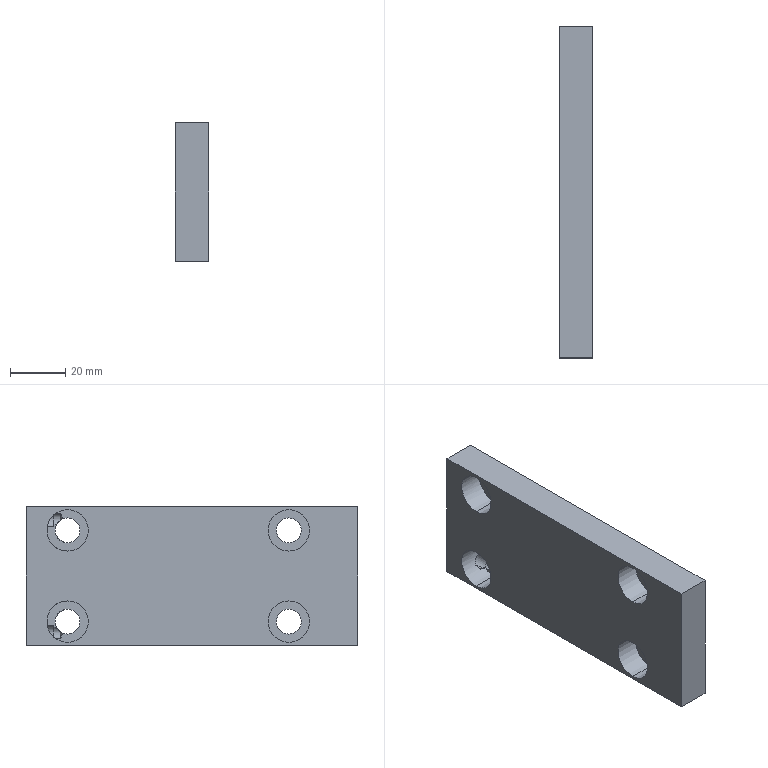Part | STEP file | X77-04102 | 1 solid | 37 faces | box 12 x 120 x 50 mm | volume 64489 mm3 | cylinder 23 | plane 12 | cone 2 | commonest cylinder face diameters 9 x8 15 x8 5 x4 4.2 x3
STEP:
#1=CARTESIAN_POINT('',(7.392,92.45,43.));
#2=VERTEX_POINT('',#1);
#3=CARTESIAN_POINT('',(5.462,90.102,47.09));
#4=VERTEX_POINT('',#3);
#5=CARTESIAN_POINT('',(7.392,92.45,43.));
#6=CARTESIAN_POINT('',(7.13,92.45,43.));
#7=CARTESIAN_POINT('',(6.865,92.442,43.042));
#8=CARTESIAN_POINT('',(6.369,92.406,43.204));
#9=CARTESIAN_POINT('',(6.131,92.378,43.325));
#10=CARTESIAN_POINT('',(5.714,92.295,43.629));
#11=CARTESIAN_POINT('',(5.528,92.239,43.815));
#12=CARTESIAN_POINT('',(5.23,92.095,44.219));
#13=CARTESIAN_POINT('',(5.113,92.005,44.443));
#14=CARTESIAN_POINT('',(4.954,91.794,44.895));
#15=CARTESIAN_POINT('',(4.909,91.671,45.128));
#16=CARTESIAN_POINT('',(4.883,91.402,45.577));
#17=CARTESIAN_POINT('',(4.9,91.254,45.797));
#18=CARTESIAN_POINT('',(4.986,90.943,46.211));
#19=CARTESIAN_POINT('',(5.052,90.782,46.404));
#20=CARTESIAN_POINT('',(5.227,90.447,46.767));
#21=CARTESIAN_POINT('',(5.335,90.274,46.936));
#22=CARTESIAN_POINT('',(5.462,90.102,47.09));
#23=B_SPLINE_CURVE_WITH_KNOTS('',3,(#5,#6,#7,#8,#9,#10,#11,#12,#13,#14,#15,#16,#17,#18,#19,#20,#21,#22),.UNSPECIFIED.,.F.,.F.,(4,2,2,2,2,2,2,2,4),(0.0005016,0.001286,0.00207,0.002854,0.003638,0.004422,0.005206,0.00599,0.006774),.UNSPECIFIED.);
#24=EDGE_CURVE('',#2,#4,#23,.T.);
#25=ORIENTED_EDGE('',*,*,#24,.F.);
#26=CARTESIAN_POINT('',(7.392,100.102,43.));
#27=VERTEX_POINT('',#26);
#28=CARTESIAN_POINT('',(7.392,100.102,43.));
#29=DIRECTION('',(0.,1.,0.));
#30=VECTOR('',#29,1000.);
#31=LINE('',#28,#30);
#32=EDGE_CURVE('',#2,#27,#31,.T.);
#33=ORIENTED_EDGE('',*,*,#32,.T.);
#34=CARTESIAN_POINT('',(7.392,100.102,48.));
#35=VERTEX_POINT('',#34);
#36=CARTESIAN_POINT('',(7.392,100.102,45.5));
#37=DIRECTION('',(0.,1.,0.));
#38=DIRECTION('',(0.,0.,1.));
#39=AXIS2_PLACEMENT_3D('',#36,#37,#38);
#40=CIRCLE('',#39,2.5);
#41=EDGE_CURVE('',#27,#35,#40,.T.);
#42=ORIENTED_EDGE('',*,*,#41,.T.);
#43=CARTESIAN_POINT('',(7.392,90.102,48.));
#44=VERTEX_POINT('',#43);
#45=CARTESIAN_POINT('',(7.392,100.102,48.));
#46=DIRECTION('',(0.,1.,0.));
#47=VECTOR('',#46,1000.);
#48=LINE('',#45,#47);
#49=EDGE_CURVE('',#44,#35,#48,.T.);
#50=ORIENTED_EDGE('',*,*,#49,.F.);
#51=CARTESIAN_POINT('',(7.392,90.102,45.5));
#52=DIRECTION('',(0.,1.,0.));
#53=DIRECTION('',(0.,0.,1.));
#54=AXIS2_PLACEMENT_3D('',#51,#52,#53);
#55=CIRCLE('',#54,2.5);
#56=EDGE_CURVE('',#4,#44,#55,.T.);
#57=ORIENTED_EDGE('',*,*,#56,.F.);
#58=EDGE_LOOP('',(#25,#33,#42,#50,#57));
#59=FACE_OUTER_BOUND('',#58,.T.);
#60=CARTESIAN_POINT('',(7.392,100.102,45.5));
#61=DIRECTION('',(0.,1.,0.));
#62=DIRECTION('',(0.,0.,1.));
#63=AXIS2_PLACEMENT_3D('',#60,#61,#62);
#64=CYLINDRICAL_SURFACE('',#63,2.5);
#65=ADVANCED_FACE('',(#59),#64,.F.);
#66=CARTESIAN_POINT('',(7.392,89.465,47.6));
#67=VERTEX_POINT('',#66);
#68=CARTESIAN_POINT('',(7.892,89.549,47.54));
#69=VERTEX_POINT('',#68);
#70=CARTESIAN_POINT('',(7.392,89.465,47.6));
#71=CARTESIAN_POINT('',(7.564,89.465,47.6));
#72=CARTESIAN_POINT('',(7.732,89.495,47.579));
#73=CARTESIAN_POINT('',(7.892,89.549,47.54));
#74=B_SPLINE_CURVE_WITH_KNOTS('',3,(#70,#71,#72,#73),.UNSPECIFIED.,.F.,.F.,(4,4),(0.001644,0.002153),.UNSPECIFIED.);
#75=EDGE_CURVE('',#67,#69,#74,.T.);
#76=ORIENTED_EDGE('',*,*,#75,.F.);
#77=CARTESIAN_POINT('',(7.392,90.102,47.6));
#78=VERTEX_POINT('',#77);
#79=CARTESIAN_POINT('',(7.392,100.102,47.6));
#80=DIRECTION('',(0.,1.,0.));
#81=VECTOR('',#80,1000.);
#82=LINE('',#79,#81);
#83=EDGE_CURVE('',#67,#78,#82,.T.);
#84=ORIENTED_EDGE('',*,*,#83,.T.);
#85=CARTESIAN_POINT('',(7.892,90.102,43.46));
#86=VERTEX_POINT('',#85);
#87=CARTESIAN_POINT('',(7.392,90.102,45.5));
#88=DIRECTION('',(0.,1.,0.));
#89=DIRECTION('',(0.,0.,1.));
#90=AXIS2_PLACEMENT_3D('',#87,#88,#89);
#91=CIRCLE('',#90,2.1);
#92=EDGE_CURVE('',#78,#86,#91,.T.);
#93=ORIENTED_EDGE('',*,*,#92,.T.);
#94=CARTESIAN_POINT('',(7.892,89.152,43.46));
#95=VERTEX_POINT('',#94);
#96=CARTESIAN_POINT('',(7.892,100.102,43.46));
#97=DIRECTION('',(0.,1.,0.));
#98=VECTOR('',#97,1000.);
#99=LINE('',#96,#98);
#100=EDGE_CURVE('',#95,#86,#99,.T.);
#101=ORIENTED_EDGE('',*,*,#100,.F.);
#102=CARTESIAN_POINT('',(9.466,87.702,45.173));
#103=VERTEX_POINT('',#102);
#104=CARTESIAN_POINT('',(9.466,87.702,45.173));
#105=CARTESIAN_POINT('',(9.443,87.903,45.031));
#106=CARTESIAN_POINT('',(9.404,88.087,44.875));
#107=CARTESIAN_POINT('',(9.271,88.422,44.547));
#108=CARTESIAN_POINT('',(9.174,88.574,44.37));
#109=CARTESIAN_POINT('',(8.914,88.824,44.038));
#110=CARTESIAN_POINT('',(8.746,88.925,43.879));
#111=CARTESIAN_POINT('',(8.358,89.074,43.621));
#112=CARTESIAN_POINT('',(8.132,89.124,43.519));
#113=CARTESIAN_POINT('',(7.892,89.152,43.46));
#114=B_SPLINE_CURVE_WITH_KNOTS('',3,(#104,#105,#106,#107,#108,#109,#110,#111,#112,#113),.UNSPECIFIED.,.F.,.F.,(4,2,2,2,4),(0.,0.0007303,0.001461,0.002191,0.002921),.UNSPECIFIED.);
#115=EDGE_CURVE('',#103,#95,#114,.T.);
#116=ORIENTED_EDGE('',*,*,#115,.F.);
#117=CARTESIAN_POINT('',(7.892,87.702,47.54));
#118=VERTEX_POINT('',#117);
#119=CARTESIAN_POINT('',(7.392,87.702,45.5));
#120=DIRECTION('',(0.,1.,0.));
#121=DIRECTION('',(0.,0.,1.));
#122=AXIS2_PLACEMENT_3D('',#119,#120,#121);
#123=CIRCLE('',#122,2.1);
#124=EDGE_CURVE('',#118,#103,#123,.T.);
#125=ORIENTED_EDGE('',*,*,#124,.F.);
#126=CARTESIAN_POINT('',(7.892,100.102,47.54));
#127=DIRECTION('',(0.,-1.,0.));
#128=VECTOR('',#127,1000.);
#129=LINE('',#126,#128);
#130=EDGE_CURVE('',#69,#118,#129,.T.);
#131=ORIENTED_EDGE('',*,*,#130,.F.);
#132=EDGE_LOOP('',(#76,#84,#93,#101,#116,#125,#131));
#133=FACE_OUTER_BOUND('',#132,.T.);
#134=CARTESIAN_POINT('',(7.392,100.102,45.5));
#135=DIRECTION('',(0.,1.,0.));
#136=DIRECTION('',(0.,0.,1.));
#137=AXIS2_PLACEMENT_3D('',#134,#135,#136);
#138=CYLINDRICAL_SURFACE('',#137,2.1);
#139=ADVANCED_FACE('',(#133),#138,.F.);
#140=CARTESIAN_POINT('',(7.392,90.102,2.));
#141=VERTEX_POINT('',#140);
#142=CARTESIAN_POINT('',(5.462,90.102,2.91));
#143=VERTEX_POINT('',#142);
#144=CARTESIAN_POINT('',(7.392,90.102,4.5));
#145=DIRECTION('',(0.,1.,0.));
#146=DIRECTION('',(0.,0.,1.));
#147=AXIS2_PLACEMENT_3D('',#144,#145,#146);
#148=CIRCLE('',#147,2.5);
#149=EDGE_CURVE('',#141,#143,#148,.T.);
#150=ORIENTED_EDGE('',*,*,#149,.F.);
#151=CARTESIAN_POINT('',(7.392,100.102,2.));
#152=VERTEX_POINT('',#151);
#153=CARTESIAN_POINT('',(7.392,100.102,2.));
#154=DIRECTION('',(0.,1.,0.));
#155=VECTOR('',#154,1000.);
#156=LINE('',#153,#155);
#157=EDGE_CURVE('',#141,#152,#156,.T.);
#158=ORIENTED_EDGE('',*,*,#157,.T.);
#159=CARTESIAN_POINT('',(7.392,100.102,7.));
#160=VERTEX_POINT('',#159);
#161=CARTESIAN_POINT('',(7.392,100.102,4.5));
#162=DIRECTION('',(0.,1.,0.));
#163=DIRECTION('',(0.,0.,1.));
#164=AXIS2_PLACEMENT_3D('',#161,#162,#163);
#165=CIRCLE('',#164,2.5);
#166=EDGE_CURVE('',#152,#160,#165,.T.);
#167=ORIENTED_EDGE('',*,*,#166,.T.);
#168=CARTESIAN_POINT('',(7.392,92.45,7.));
#169=VERTEX_POINT('',#168);
#170=CARTESIAN_POINT('',(7.392,100.102,7.));
#171=DIRECTION('',(0.,1.,0.));
#172=VECTOR('',#171,1000.);
#173=LINE('',#170,#172);
#174=EDGE_CURVE('',#169,#160,#173,.T.);
#175=ORIENTED_EDGE('',*,*,#174,.F.);
#176=CARTESIAN_POINT('',(5.462,90.102,2.91));
#177=CARTESIAN_POINT('',(5.335,90.274,3.064));
#178=CARTESIAN_POINT('',(5.228,90.445,3.231));
#179=CARTESIAN_POINT('',(5.053,90.779,3.593));
#180=CARTESIAN_POINT('',(4.985,90.945,3.79));
#181=CARTESIAN_POINT('',(4.9,91.255,4.204));
#182=CARTESIAN_POINT('',(4.883,91.401,4.42));
#183=CARTESIAN_POINT('',(4.909,91.672,4.873));
#184=CARTESIAN_POINT('',(4.953,91.793,5.102));
#185=CARTESIAN_POINT('',(5.073,91.952,5.443));
#186=CARTESIAN_POINT('',(5.122,92.001,5.557));
#187=CARTESIAN_POINT('',(5.237,92.09,5.775));
#188=CARTESIAN_POINT('',(5.303,92.13,5.88));
#189=CARTESIAN_POINT('',(5.526,92.238,6.183));
#190=CARTESIAN_POINT('',(5.712,92.295,6.37));
#191=CARTESIAN_POINT('',(6.13,92.378,6.674));
#192=CARTESIAN_POINT('',(6.368,92.406,6.796));
#193=CARTESIAN_POINT('',(6.865,92.442,6.958));
#194=CARTESIAN_POINT('',(7.13,92.45,7.));
#195=CARTESIAN_POINT('',(7.392,92.45,7.));
#196=B_SPLINE_CURVE_WITH_KNOTS('',3,(#176,#177,#178,#179,#180,#181,#182,#183,#184,#185,#186,#187,#188,#189,#190,#191,#192,#193,#194,#195),.UNSPECIFIED.,.F.,.F.,(4,2,2,2,2,2,2,2,2,4),(0.,0.0007837,0.001567,0.002351,0.003135,0.003526,0.003918,0.004702,0.005486,0.006269),.UNSPECIFIED.);
#197=EDGE_CURVE('',#143,#169,#196,.T.);
#198=ORIENTED_EDGE('',*,*,#197,.F.);
#199=EDGE_LOOP('',(#150,#158,#167,#175,#198));
#200=FACE_OUTER_BOUND('',#199,.T.);
#201=CARTESIAN_POINT('',(7.392,100.102,4.5));
#202=DIRECTION('',(0.,1.,0.));
#203=DIRECTION('',(0.,0.,1.));
#204=AXIS2_PLACEMENT_3D('',#201,#202,#203);
#205=CYLINDRICAL_SURFACE('',#204,2.5);
#206=ADVANCED_FACE('',(#200),#205,.F.);
#207=CARTESIAN_POINT('',(7.892,5.102,34.));
#208=VERTEX_POINT('',#207);
#209=CARTESIAN_POINT('',(7.892,5.102,49.));
#210=VERTEX_POINT('',#209);
#211=CARTESIAN_POINT('',(7.892,5.102,41.5));
#212=DIRECTION('',(-1.,0.,0.));
#213=DIRECTION('',(0.,0.,1.));
#214=AXIS2_PLACEMENT_3D('',#211,#212,#213);
#215=CIRCLE('',#214,7.5);
#216=EDGE_CURVE('',#208,#210,#215,.T.);
#217=ORIENTED_EDGE('',*,*,#216,.F.);
#218=CARTESIAN_POINT('',(-1.108,5.102,34.));
#219=VERTEX_POINT('',#218);
#220=CARTESIAN_POINT('',(-1.108,5.102,34.));
#221=DIRECTION('',(-1.,0.,0.));
#222=VECTOR('',#221,1000.);
#223=LINE('',#220,#222);
#224=EDGE_CURVE('',#208,#219,#223,.T.);
#225=ORIENTED_EDGE('',*,*,#224,.T.);
#226=CARTESIAN_POINT('',(-1.108,5.102,49.));
#227=VERTEX_POINT('',#226);
#228=CARTESIAN_POINT('',(-1.108,5.102,41.5));
#229=DIRECTION('',(-1.,0.,0.));
#230=DIRECTION('',(0.,0.,1.));
#231=AXIS2_PLACEMENT_3D('',#228,#229,#230);
#232=CIRCLE('',#231,7.5);
#233=EDGE_CURVE('',#219,#227,#232,.T.);
#234=ORIENTED_EDGE('',*,*,#233,.T.);
#235=CARTESIAN_POINT('',(-1.108,5.102,49.));
#236=DIRECTION('',(-1.,0.,0.));
#237=VECTOR('',#236,1000.);
#238=LINE('',#235,#237);
#239=EDGE_CURVE('',#210,#227,#238,.T.);
#240=ORIENTED_EDGE('',*,*,#239,.F.);
#241=EDGE_LOOP('',(#217,#225,#234,#240));
#242=FACE_OUTER_BOUND('',#241,.T.);
#243=CARTESIAN_POINT('',(-1.108,5.102,41.5));
#244=DIRECTION('',(-1.,0.,0.));
#245=DIRECTION('',(0.,0.,1.));
#246=AXIS2_PLACEMENT_3D('',#243,#244,#245);
#247=CYLINDRICAL_SURFACE('',#246,7.5);
#248=ADVANCED_FACE('',(#242),#247,.F.);
#249=CARTESIAN_POINT('',(10.892,5.102,37.));
#250=VERTEX_POINT('',#249);
#251=CARTESIAN_POINT('',(10.892,5.102,46.));
#252=VERTEX_POINT('',#251);
#253=CARTESIAN_POINT('',(10.892,5.102,41.5));
#254=DIRECTION('',(-1.,0.,0.));
#255=DIRECTION('',(0.,-1.,0.));
#256=AXIS2_PLACEMENT_3D('',#253,#254,#255);
#257=CIRCLE('',#256,4.5);
#258=EDGE_CURVE('',#250,#252,#257,.T.);
#259=ORIENTED_EDGE('',*,*,#258,.F.);
#260=CARTESIAN_POINT('',(7.892,5.102,37.));
#261=VERTEX_POINT('',#260);
#262=CARTESIAN_POINT('',(-1.108,5.102,37.));
#263=DIRECTION('',(-1.,0.,0.));
#264=VECTOR('',#263,1000.);
#265=LINE('',#262,#264);
#266=EDGE_CURVE('',#250,#261,#265,.T.);
#267=ORIENTED_EDGE('',*,*,#266,.T.);
#268=CARTESIAN_POINT('',(7.892,5.102,46.));
#269=VERTEX_POINT('',#268);
#270=CARTESIAN_POINT('',(7.892,5.102,41.5));
#271=DIRECTION('',(-1.,0.,0.));
#272=DIRECTION('',(0.,0.,1.));
#273=AXIS2_PLACEMENT_3D('',#270,#271,#272);
#274=CIRCLE('',#273,4.5);
#275=EDGE_CURVE('',#261,#269,#274,.T.);
#276=ORIENTED_EDGE('',*,*,#275,.T.);
#277=CARTESIAN_POINT('',(-1.108,5.102,46.));
#278=DIRECTION('',(-1.,0.,0.));
#279=VECTOR('',#278,1000.);
#280=LINE('',#277,#279);
#281=EDGE_CURVE('',#252,#269,#280,.T.);
#282=ORIENTED_EDGE('',*,*,#281,.F.);
#283=EDGE_LOOP('',(#259,#267,#276,#282));
#284=FACE_OUTER_BOUND('',#283,.T.);
#285=CARTESIAN_POINT('',(-1.108,5.102,41.5));
#286=DIRECTION('',(-1.,0.,0.));
#287=DIRECTION('',(0.,0.,1.));
#288=AXIS2_PLACEMENT_3D('',#285,#286,#287);
#289=CYLINDRICAL_SURFACE('',#288,4.5);
#290=ADVANCED_FACE('',(#284),#289,.F.);
#291=CARTESIAN_POINT('',(7.892,85.102,34.));
#292=VERTEX_POINT('',#291);
#293=CARTESIAN_POINT('',(7.892,85.102,49.));
#294=VERTEX_POINT('',#293);
#295=CARTESIAN_POINT('',(7.892,85.102,41.5));
#296=DIRECTION('',(-1.,0.,0.));
#297=DIRECTION('',(0.,0.,1.));
#298=AXIS2_PLACEMENT_3D('',#295,#296,#297);
#299=CIRCLE('',#298,7.5);
#300=EDGE_CURVE('',#292,#294,#299,.T.);
#301=ORIENTED_EDGE('',*,*,#300,.F.);
#302=CARTESIAN_POINT('',(-1.108,85.102,34.));
#303=VERTEX_POINT('',#302);
#304=CARTESIAN_POINT('',(-1.108,85.102,34.));
#305=DIRECTION('',(-1.,0.,0.));
#306=VECTOR('',#305,1000.);
#307=LINE('',#304,#306);
#308=EDGE_CURVE('',#292,#303,#307,.T.);
#309=ORIENTED_EDGE('',*,*,#308,.T.);
#310=CARTESIAN_POINT('',(-1.108,85.102,49.));
#311=VERTEX_POINT('',#310);
#312=CARTESIAN_POINT('',(-1.108,85.102,41.5));
#313=DIRECTION('',(-1.,0.,0.));
#314=DIRECTION('',(0.,0.,1.));
#315=AXIS2_PLACEMENT_3D('',#312,#313,#314);
#316=CIRCLE('',#315,7.5);
#317=EDGE_CURVE('',#303,#311,#316,.T.);
#318=ORIENTED_EDGE('',*,*,#317,.T.);
#319=CARTESIAN_POINT('',(-1.108,85.102,49.));
#320=DIRECTION('',(-1.,0.,0.));
#321=VECTOR('',#320,1000.);
#322=LINE('',#319,#321);
#323=EDGE_CURVE('',#294,#311,#322,.T.);
#324=ORIENTED_EDGE('',*,*,#323,.F.);
#325=EDGE_LOOP('',(#301,#309,#318,#324));
#326=FACE_OUTER_BOUND('',#325,.T.);
#327=CARTESIAN_POINT('',(-1.108,85.102,41.5));
#328=DIRECTION('',(-1.,0.,0.));
#329=DIRECTION('',(0.,0.,1.));
#330=AXIS2_PLACEMENT_3D('',#327,#328,#329);
#331=CYLINDRICAL_SURFACE('',#330,7.5);
#332=ADVANCED_FACE('',(#326),#331,.F.);
#333=CARTESIAN_POINT('',(10.892,85.102,37.));
#334=VERTEX_POINT('',#333);
#335=CARTESIAN_POINT('',(10.892,85.102,46.));
#336=VERTEX_POINT('',#335);
#337=CARTESIAN_POINT('',(10.892,85.102,41.5));
#338=DIRECTION('',(-1.,0.,0.));
#339=DIRECTION('',(0.,-1.,0.));
#340=AXIS2_PLACEMENT_3D('',#337,#338,#339);
#341=CIRCLE('',#340,4.5);
#342=EDGE_CURVE('',#334,#336,#341,.T.);
#343=ORIENTED_EDGE('',*,*,#342,.F.);
#344=CARTESIAN_POINT('',(7.892,85.102,37.));
#345=VERTEX_POINT('',#344);
#346=CARTESIAN_POINT('',(-1.108,85.102,37.));
#347=DIRECTION('',(-1.,0.,0.));
#348=VECTOR('',#347,1000.);
#349=LINE('',#346,#348);
#350=EDGE_CURVE('',#334,#345,#349,.T.);
#351=ORIENTED_EDGE('',*,*,#350,.T.);
#352=CARTESIAN_POINT('',(7.892,85.102,46.));
#353=VERTEX_POINT('',#352);
#354=CARTESIAN_POINT('',(7.892,85.102,41.5));
#355=DIRECTION('',(-1.,0.,0.));
#356=DIRECTION('',(0.,0.,1.));
#357=AXIS2_PLACEMENT_3D('',#354,#355,#356);
#358=CIRCLE('',#357,4.5);
#359=EDGE_CURVE('',#345,#353,#358,.T.);
#360=ORIENTED_EDGE('',*,*,#359,.T.);
#361=CARTESIAN_POINT('',(-1.108,85.102,46.));
#362=DIRECTION('',(-1.,0.,0.));
#363=VECTOR('',#362,1000.);
#364=LINE('',#361,#363);
#365=EDGE_CURVE('',#336,#353,#364,.T.);
#366=ORIENTED_EDGE('',*,*,#365,.F.);
#367=EDGE_LOOP('',(#343,#351,#360,#366));
#368=FACE_OUTER_BOUND('',#367,.T.);
#369=CARTESIAN_POINT('',(-1.108,85.102,41.5));
#370=DIRECTION('',(-1.,0.,0.));
#371=DIRECTION('',(0.,0.,1.));
#372=AXIS2_PLACEMENT_3D('',#369,#370,#371);
#373=CYLINDRICAL_SURFACE('',#372,4.5);
#374=ADVANCED_FACE('',(#368),#373,.F.);
#375=CARTESIAN_POINT('',(7.892,5.102,1.));
#376=VERTEX_POINT('',#375);
#377=CARTESIAN_POINT('',(7.892,5.102,16.));
#378=VERTEX_POINT('',#377);
#379=CARTESIAN_POINT('',(7.892,5.102,8.5));
#380=DIRECTION('',(-1.,0.,0.));
#381=DIRECTION('',(0.,0.,1.));
#382=AXIS2_PLACEMENT_3D('',#379,#380,#381);
#383=CIRCLE('',#382,7.5);
#384=EDGE_CURVE('',#376,#378,#383,.T.);
#385=ORIENTED_EDGE('',*,*,#384,.F.);
#386=CARTESIAN_POINT('',(-1.108,5.102,1.));
#387=VERTEX_POINT('',#386);
#388=CARTESIAN_POINT('',(-1.108,5.102,1.));
#389=DIRECTION('',(-1.,0.,0.));
#390=VECTOR('',#389,1000.);
#391=LINE('',#388,#390);
#392=EDGE_CURVE('',#376,#387,#391,.T.);
#393=ORIENTED_EDGE('',*,*,#392,.T.);
#394=CARTESIAN_POINT('',(-1.108,5.102,16.));
#395=VERTEX_POINT('',#394);
#396=CARTESIAN_POINT('',(-1.108,5.102,8.5));
#397=DIRECTION('',(-1.,0.,0.));
#398=DIRECTION('',(0.,0.,1.));
#399=AXIS2_PLACEMENT_3D('',#396,#397,#398);
#400=CIRCLE('',#399,7.5);
#401=EDGE_CURVE('',#387,#395,#400,.T.);
#402=ORIENTED_EDGE('',*,*,#401,.T.);
#403=CARTESIAN_POINT('',(-1.108,5.102,16.));
#404=DIRECTION('',(-1.,0.,0.));
#405=VECTOR('',#404,1000.);
#406=LINE('',#403,#405);
#407=EDGE_CURVE('',#378,#395,#406,.T.);
#408=ORIENTED_EDGE('',*,*,#407,.F.);
#409=EDGE_LOOP('',(#385,#393,#402,#408));
#410=FACE_OUTER_BOUND('',#409,.T.);
#411=CARTESIAN_POINT('',(-1.108,5.102,8.5));
#412=DIRECTION('',(-1.,0.,0.));
#413=DIRECTION('',(0.,0.,1.));
#414=AXIS2_PLACEMENT_3D('',#411,#412,#413);
#415=CYLINDRICAL_SURFACE('',#414,7.5);
#416=ADVANCED_FACE('',(#410),#415,.F.);
#417=CARTESIAN_POINT('',(10.892,5.102,4.));
#418=VERTEX_POINT('',#417);
#419=CARTESIAN_POINT('',(10.892,5.102,13.));
#420=VERTEX_POINT('',#419);
#421=CARTESIAN_POINT('',(10.892,5.102,8.5));
#422=DIRECTION('',(-1.,0.,0.));
#423=DIRECTION('',(0.,-1.,0.));
#424=AXIS2_PLACEMENT_3D('',#421,#422,#423);
#425=CIRCLE('',#424,4.5);
#426=EDGE_CURVE('',#418,#420,#425,.T.);
#427=ORIENTED_EDGE('',*,*,#426,.F.);
#428=CARTESIAN_POINT('',(7.892,5.102,4.));
#429=VERTEX_POINT('',#428);
#430=CARTESIAN_POINT('',(-1.108,5.102,4.));
#431=DIRECTION('',(-1.,0.,0.));
#432=VECTOR('',#431,1000.);
#433=LINE('',#430,#432);
#434=EDGE_CURVE('',#418,#429,#433,.T.);
#435=ORIENTED_EDGE('',*,*,#434,.T.);
#436=CARTESIAN_POINT('',(7.892,5.102,13.));
#437=VERTEX_POINT('',#436);
#438=CARTESIAN_POINT('',(7.892,5.102,8.5));
#439=DIRECTION('',(-1.,0.,0.));
#440=DIRECTION('',(0.,0.,1.));
#441=AXIS2_PLACEMENT_3D('',#438,#439,#440);
#442=CIRCLE('',#441,4.5);
#443=EDGE_CURVE('',#429,#437,#442,.T.);
#444=ORIENTED_EDGE('',*,*,#443,.T.);
#445=CARTESIAN_POINT('',(-1.108,5.102,13.));
#446=DIRECTION('',(-1.,0.,0.));
#447=VECTOR('',#446,1000.);
#448=LINE('',#445,#447);
#449=EDGE_CURVE('',#420,#437,#448,.T.);
#450=ORIENTED_EDGE('',*,*,#449,.F.);
#451=EDGE_LOOP('',(#427,#435,#444,#450));
#452=FACE_OUTER_BOUND('',#451,.T.);
#453=CARTESIAN_POINT('',(-1.108,5.102,8.5));
#454=DIRECTION('',(-1.,0.,0.));
#455=DIRECTION('',(0.,0.,1.));
#456=AXIS2_PLACEMENT_3D('',#453,#454,#455);
#457=CYLINDRICAL_SURFACE('',#456,4.5);
#458=ADVANCED_FACE('',(#452),#457,.F.);
#459=CARTESIAN_POINT('',(7.892,85.102,1.));
#460=VERTEX_POINT('',#459);
#461=CARTESIAN_POINT('',(7.892,85.102,16.));
#462=VERTEX_POINT('',#461);
#463=CARTESIAN_POINT('',(7.892,85.102,8.5));
#464=DIRECTION('',(-1.,0.,0.));
#465=DIRECTION('',(0.,0.,1.));
#466=AXIS2_PLACEMENT_3D('',#463,#464,#465);
#467=CIRCLE('',#466,7.5);
#468=EDGE_CURVE('',#460,#462,#467,.T.);
#469=ORIENTED_EDGE('',*,*,#468,.F.);
#470=CARTESIAN_POINT('',(-1.108,85.102,1.));
#471=VERTEX_POINT('',#470);
#472=CARTESIAN_POINT('',(-1.108,85.102,1.));
#473=DIRECTION('',(-1.,0.,0.));
#474=VECTOR('',#473,1000.);
#475=LINE('',#472,#474);
#476=EDGE_CURVE('',#460,#471,#475,.T.);
#477=ORIENTED_EDGE('',*,*,#476,.T.);
#478=CARTESIAN_POINT('',(-1.108,85.102,16.));
#479=VERTEX_POINT('',#478);
#480=CARTESIAN_POINT('',(-1.108,85.102,8.5));
#481=DIRECTION('',(-1.,0.,0.));
#482=DIRECTION('',(0.,0.,1.));
#483=AXIS2_PLACEMENT_3D('',#480,#481,#482);
#484=CIRCLE('',#483,7.5);
#485=EDGE_CURVE('',#471,#479,#484,.T.);
#486=ORIENTED_EDGE('',*,*,#485,.T.);
#487=CARTESIAN_POINT('',(-1.108,85.102,16.));
#488=DIRECTION('',(-1.,0.,0.));
#489=VECTOR('',#488,1000.);
#490=LINE('',#487,#489);
#491=EDGE_CURVE('',#462,#479,#490,.T.);
#492=ORIENTED_EDGE('',*,*,#491,.F.);
#493=EDGE_LOOP('',(#469,#477,#486,#492));
#494=FACE_OUTER_BOUND('',#493,.T.);
#495=CARTESIAN_POINT('',(-1.108,85.102,8.5));
#496=DIRECTION('',(-1.,0.,0.));
#497=DIRECTION('',(0.,0.,1.));
#498=AXIS2_PLACEMENT_3D('',#495,#496,#497);
#499=CYLINDRICAL_SURFACE('',#498,7.5);
#500=ADVANCED_FACE('',(#494),#499,.F.);
#501=CARTESIAN_POINT('',(10.892,85.102,4.));
#502=VERTEX_POINT('',#501);
#503=CARTESIAN_POINT('',(10.892,85.102,13.));
#504=VERTEX_POINT('',#503);
#505=CARTESIAN_POINT('',(10.892,85.102,8.5));
#506=DIRECTION('',(-1.,0.,0.));
#507=DIRECTION('',(0.,-1.,0.));
#508=AXIS2_PLACEMENT_3D('',#505,#506,#507);
#509=CIRCLE('',#508,4.5);
#510=EDGE_CURVE('',#502,#504,#509,.T.);
#511=ORIENTED_EDGE('',*,*,#510,.F.);
#512=CARTESIAN_POINT('',(7.892,85.102,4.));
#513=VERTEX_POINT('',#512);
#514=CARTESIAN_POINT('',(-1.108,85.102,4.));
#515=DIRECTION('',(-1.,0.,0.));
#516=VECTOR('',#515,1000.);
#517=LINE('',#514,#516);
#518=EDGE_CURVE('',#502,#513,#517,.T.);
#519=ORIENTED_EDGE('',*,*,#518,.T.);
#520=CARTESIAN_POINT('',(7.892,85.102,13.));
#521=VERTEX_POINT('',#520);
#522=CARTESIAN_POINT('',(7.892,85.102,8.5));
#523=DIRECTION('',(-1.,0.,0.));
#524=DIRECTION('',(0.,0.,1.));
#525=AXIS2_PLACEMENT_3D('',#522,#523,#524);
#526=CIRCLE('',#525,4.5);
#527=EDGE_CURVE('',#513,#521,#526,.T.);
#528=ORIENTED_EDGE('',*,*,#527,.T.);
#529=CARTESIAN_POINT('',(-1.108,85.102,13.));
#530=DIRECTION('',(-1.,0.,0.));
#531=VECTOR('',#530,1000.);
#532=LINE('',#529,#531);
#533=EDGE_CURVE('',#504,#521,#532,.T.);
#534=ORIENTED_EDGE('',*,*,#533,.F.);
#535=EDGE_LOOP('',(#511,#519,#528,#534));
#536=FACE_OUTER_BOUND('',#535,.T.);
#537=CARTESIAN_POINT('',(-1.108,85.102,8.5));
#538=DIRECTION('',(-1.,0.,0.));
#539=DIRECTION('',(0.,0.,1.));
#540=AXIS2_PLACEMENT_3D('',#537,#538,#539);
#541=CYLINDRICAL_SURFACE('',#540,4.5);
#542=ADVANCED_FACE('',(#536),#541,.F.);
#543=CARTESIAN_POINT('',(-1.108,5.102,41.5));
#544=DIRECTION('',(-1.,0.,0.));
#545=DIRECTION('',(0.,0.,1.));
#546=AXIS2_PLACEMENT_3D('',#543,#544,#545);
#547=CIRCLE('',#546,7.5);
#548=EDGE_CURVE('',#227,#219,#547,.T.);
#549=ORIENTED_EDGE('',*,*,#548,.F.);
#550=ORIENTED_EDGE('',*,*,#233,.F.);
#551=EDGE_LOOP('',(#549,#550));
#552=FACE_BOUND('',#551,.T.);
#553=CARTESIAN_POINT('',(-1.108,85.102,41.5));
#554=DIRECTION('',(-1.,0.,0.));
#555=DIRECTION('',(0.,0.,1.));
#556=AXIS2_PLACEMENT_3D('',#553,#554,#555);
#557=CIRCLE('',#556,7.5);
#558=EDGE_CURVE('',#311,#303,#557,.T.);
#559=ORIENTED_EDGE('',*,*,#558,.F.);
#560=ORIENTED_EDGE('',*,*,#317,.F.);
#561=EDGE_LOOP('',(#559,#560));
#562=FACE_BOUND('',#561,.T.);
#563=CARTESIAN_POINT('',(-1.108,5.102,8.5));
#564=DIRECTION('',(-1.,0.,0.));
#565=DIRECTION('',(0.,0.,1.));
#566=AXIS2_PLACEMENT_3D('',#563,#564,#565);
#567=CIRCLE('',#566,7.5);
#568=EDGE_CURVE('',#395,#387,#567,.T.);
#569=ORIENTED_EDGE('',*,*,#568,.F.);
#570=ORIENTED_EDGE('',*,*,#401,.F.);
#571=EDGE_LOOP('',(#569,#570));
#572=FACE_BOUND('',#571,.T.);
#573=CARTESIAN_POINT('',(-1.108,85.102,8.5));
#574=DIRECTION('',(-1.,0.,0.));
#575=DIRECTION('',(0.,0.,1.));
#576=AXIS2_PLACEMENT_3D('',#573,#574,#575);
#577=CIRCLE('',#576,7.5);
#578=EDGE_CURVE('',#479,#471,#577,.T.);
#579=ORIENTED_EDGE('',*,*,#578,.F.);
#580=ORIENTED_EDGE('',*,*,#485,.F.);
#581=EDGE_LOOP('',(#579,#580));
#582=FACE_BOUND('',#581,.T.);
#583=CARTESIAN_POINT('',(-1.108,100.102,0.));
#584=VERTEX_POINT('',#583);
#585=CARTESIAN_POINT('',(-1.108,-19.898,0.));
#586=VERTEX_POINT('',#585);
#587=CARTESIAN_POINT('',(-1.108,100.102,0.));
#588=DIRECTION('',(0.,-1.,0.));
#589=VECTOR('',#588,1000.);
#590=LINE('',#587,#589);
#591=EDGE_CURVE('',#584,#586,#590,.T.);
#592=ORIENTED_EDGE('',*,*,#591,.T.);
#593=CARTESIAN_POINT('',(-1.108,-19.898,50.));
#594=VERTEX_POINT('',#593);
#595=CARTESIAN_POINT('',(-1.108,-19.898,50.));
#596=DIRECTION('',(0.,0.,-1.));
#597=VECTOR('',#596,1000.);
#598=LINE('',#595,#597);
#599=EDGE_CURVE('',#594,#586,#598,.T.);
#600=ORIENTED_EDGE('',*,*,#599,.F.);
#601=CARTESIAN_POINT('',(-1.108,100.102,50.));
#602=VERTEX_POINT('',#601);
#603=CARTESIAN_POINT('',(-1.108,100.102,50.));
#604=DIRECTION('',(0.,-1.,0.));
#605=VECTOR('',#604,1000.);
#606=LINE('',#603,#605);
#607=EDGE_CURVE('',#602,#594,#606,.T.);
#608=ORIENTED_EDGE('',*,*,#607,.F.);
#609=CARTESIAN_POINT('',(-1.108,100.102,50.));
#610=DIRECTION('',(0.,0.,-1.));
#611=VECTOR('',#610,1000.);
#612=LINE('',#609,#611);
#613=EDGE_CURVE('',#602,#584,#612,.T.);
#614=ORIENTED_EDGE('',*,*,#613,.T.);
#615=EDGE_LOOP('',(#592,#600,#608,#614));
#616=FACE_OUTER_BOUND('',#615,.T.);
#617=CARTESIAN_POINT('',(-1.108,100.102,50.));
#618=DIRECTION('',(1.,0.,0.));
#619=DIRECTION('',(0.,1.,0.));
#620=AXIS2_PLACEMENT_3D('',#617,#618,#619);
#621=PLANE('',#620);
#622=ADVANCED_FACE('',(#552,#562,#572,#582,#616),#621,.F.);
#623=CARTESIAN_POINT('',(10.892,-19.898,0.));
#624=VERTEX_POINT('',#623);
#625=CARTESIAN_POINT('',(10.892,-19.898,0.));
#626=DIRECTION('',(1.,0.,0.));
#627=VECTOR('',#626,1000.);
#628=LINE('',#625,#627);
#629=EDGE_CURVE('',#586,#624,#628,.T.);
#630=ORIENTED_EDGE('',*,*,#629,.T.);
#631=CARTESIAN_POINT('',(10.892,-19.898,50.));
#632=VERTEX_POINT('',#631);
#633=CARTESIAN_POINT('',(10.892,-19.898,50.));
#634=DIRECTION('',(0.,0.,-1.));
#635=VECTOR('',#634,1000.);
#636=LINE('',#633,#635);
#637=EDGE_CURVE('',#632,#624,#636,.T.);
#638=ORIENTED_EDGE('',*,*,#637,.F.);
#639=CARTESIAN_POINT('',(10.892,-19.898,50.));
#640=DIRECTION('',(1.,0.,0.));
#641=VECTOR('',#640,1000.);
#642=LINE('',#639,#641);
#643=EDGE_CURVE('',#594,#632,#642,.T.);
#644=ORIENTED_EDGE('',*,*,#643,.F.);
#645=ORIENTED_EDGE('',*,*,#599,.T.);
#646=EDGE_LOOP('',(#630,#638,#644,#645));
#647=FACE_OUTER_BOUND('',#646,.T.);
#648=CARTESIAN_POINT('',(10.892,-19.898,50.));
#649=DIRECTION('',(0.,1.,0.));
#650=DIRECTION('',(0.,0.,1.));
#651=AXIS2_PLACEMENT_3D('',#648,#649,#650);
#652=PLANE('',#651);
#653=ADVANCED_FACE('',(#647),#652,.F.);
#654=CARTESIAN_POINT('',(10.892,5.102,41.5));
#655=DIRECTION('',(-1.,0.,0.));
#656=DIRECTION('',(0.,-1.,0.));
#657=AXIS2_PLACEMENT_3D('',#654,#655,#656);
#658=CIRCLE('',#657,4.5);
#659=EDGE_CURVE('',#252,#250,#658,.T.);
#660=ORIENTED_EDGE('',*,*,#659,.T.);
#661=ORIENTED_EDGE('',*,*,#258,.T.);
#662=EDGE_LOOP('',(#660,#661));
#663=FACE_BOUND('',#662,.T.);
#664=CARTESIAN_POINT('',(10.892,85.102,41.5));
#665=DIRECTION('',(-1.,0.,0.));
#666=DIRECTION('',(0.,-1.,0.));
#667=AXIS2_PLACEMENT_3D('',#664,#665,#666);
#668=CIRCLE('',#667,4.5);
#669=EDGE_CURVE('',#336,#334,#668,.T.);
#670=ORIENTED_EDGE('',*,*,#669,.T.);
#671=ORIENTED_EDGE('',*,*,#342,.T.);
#672=EDGE_LOOP('',(#670,#671));
#673=FACE_BOUND('',#672,.T.);
#674=CARTESIAN_POINT('',(10.892,5.102,8.5));
#675=DIRECTION('',(-1.,0.,0.));
#676=DIRECTION('',(0.,-1.,0.));
#677=AXIS2_PLACEMENT_3D('',#674,#675,#676);
#678=CIRCLE('',#677,4.5);
#679=EDGE_CURVE('',#420,#418,#678,.T.);
#680=ORIENTED_EDGE('',*,*,#679,.T.);
#681=ORIENTED_EDGE('',*,*,#426,.T.);
#682=EDGE_LOOP('',(#680,#681));
#683=FACE_BOUND('',#682,.T.);
#684=CARTESIAN_POINT('',(10.892,85.102,8.5));
#685=DIRECTION('',(-1.,0.,0.));
#686=DIRECTION('',(0.,-1.,0.));
#687=AXIS2_PLACEMENT_3D('',#684,#685,#686);
#688=CIRCLE('',#687,4.5);
#689=EDGE_CURVE('',#504,#502,#688,.T.);
#690=ORIENTED_EDGE('',*,*,#689,.T.);
#691=ORIENTED_EDGE('',*,*,#510,.T.);
#692=EDGE_LOOP('',(#690,#691));
#693=FACE_BOUND('',#692,.T.);
#694=CARTESIAN_POINT('',(10.892,100.102,0.));
#695=VERTEX_POINT('',#694);
#696=CARTESIAN_POINT('',(10.892,100.102,0.));
#697=DIRECTION('',(0.,1.,0.));
#698=VECTOR('',#697,1000.);
#699=LINE('',#696,#698);
#700=EDGE_CURVE('',#624,#695,#699,.T.);
#701=ORIENTED_EDGE('',*,*,#700,.T.);
#702=CARTESIAN_POINT('',(10.892,100.102,50.));
#703=VERTEX_POINT('',#702);
#704=CARTESIAN_POINT('',(10.892,100.102,50.));
#705=DIRECTION('',(0.,0.,-1.));
#706=VECTOR('',#705,1000.);
#707=LINE('',#704,#706);
#708=EDGE_CURVE('',#703,#695,#707,.T.);
#709=ORIENTED_EDGE('',*,*,#708,.F.);
#710=CARTESIAN_POINT('',(10.892,100.102,50.));
#711=DIRECTION('',(0.,1.,0.));
#712=VECTOR('',#711,1000.);
#713=LINE('',#710,#712);
#714=EDGE_CURVE('',#632,#703,#713,.T.);
#715=ORIENTED_EDGE('',*,*,#714,.F.);
#716=ORIENTED_EDGE('',*,*,#637,.T.);
#717=EDGE_LOOP('',(#701,#709,#715,#716));
#718=FACE_OUTER_BOUND('',#717,.T.);
#719=CARTESIAN_POINT('',(10.892,100.102,50.));
#720=DIRECTION('',(-1.,0.,0.));
#721=DIRECTION('',(0.,-1.,0.));
#722=AXIS2_PLACEMENT_3D('',#719,#720,#721);
#723=PLANE('',#722);
#724=ADVANCED_FACE('',(#663,#673,#683,#693,#718),#723,.F.);
#725=CARTESIAN_POINT('',(7.392,100.102,45.5));
#726=DIRECTION('',(0.,1.,0.));
#727=DIRECTION('',(0.,0.,1.));
#728=AXIS2_PLACEMENT_3D('',#725,#726,#727);
#729=CIRCLE('',#728,2.5);
#730=EDGE_CURVE('',#35,#27,#729,.T.);
#731=ORIENTED_EDGE('',*,*,#730,.F.);
#732=ORIENTED_EDGE('',*,*,#41,.F.);
#733=EDGE_LOOP('',(#731,#732));
#734=FACE_BOUND('',#733,.T.);
#735=CARTESIAN_POINT('',(7.392,100.102,4.5));
#736=DIRECTION('',(0.,1.,0.));
#737=DIRECTION('',(0.,0.,1.));
#738=AXIS2_PLACEMENT_3D('',#735,#736,#737);
#739=CIRCLE('',#738,2.5);
#740=EDGE_CURVE('',#160,#152,#739,.T.);
#741=ORIENTED_EDGE('',*,*,#740,.F.);
#742=ORIENTED_EDGE('',*,*,#166,.F.);
#743=EDGE_LOOP('',(#741,#742));
#744=FACE_BOUND('',#743,.T.);
#745=CARTESIAN_POINT('',(10.892,100.102,0.));
#746=DIRECTION('',(-1.,0.,0.));
#747=VECTOR('',#746,1000.);
#748=LINE('',#745,#747);
#749=EDGE_CURVE('',#695,#584,#748,.T.);
#750=ORIENTED_EDGE('',*,*,#749,.T.);
#751=ORIENTED_EDGE('',*,*,#613,.F.);
#752=CARTESIAN_POINT('',(10.892,100.102,50.));
#753=DIRECTION('',(-1.,0.,0.));
#754=VECTOR('',#753,1000.);
#755=LINE('',#752,#754);
#756=EDGE_CURVE('',#703,#602,#755,.T.);
#757=ORIENTED_EDGE('',*,*,#756,.F.);
#758=ORIENTED_EDGE('',*,*,#708,.T.);
#759=EDGE_LOOP('',(#750,#751,#757,#758));
#760=FACE_OUTER_BOUND('',#759,.T.);
#761=CARTESIAN_POINT('',(10.892,100.102,50.));
#762=DIRECTION('',(0.,-1.,0.));
#763=DIRECTION('',(0.,0.,-1.));
#764=AXIS2_PLACEMENT_3D('',#761,#762,#763);
#765=PLANE('',#764);
#766=ADVANCED_FACE('',(#734,#744,#760),#765,.F.);
#767=ORIENTED_EDGE('',*,*,#607,.T.);
#768=ORIENTED_EDGE('',*,*,#643,.T.);
#769=ORIENTED_EDGE('',*,*,#714,.T.);
#770=ORIENTED_EDGE('',*,*,#756,.T.);
#771=EDGE_LOOP('',(#767,#768,#769,#770));
#772=FACE_OUTER_BOUND('',#771,.T.);
#773=CARTESIAN_POINT('',(-1.108,-19.898,50.));
#774=DIRECTION('',(0.,0.,-1.));
#775=DIRECTION('',(-1.,0.,0.));
#776=AXIS2_PLACEMENT_3D('',#773,#774,#775);
#777=PLANE('',#776);
#778=ADVANCED_FACE('',(#772),#777,.F.);
#779=ORIENTED_EDGE('',*,*,#591,.F.);
#780=ORIENTED_EDGE('',*,*,#749,.F.);
#781=ORIENTED_EDGE('',*,*,#700,.F.);
#782=ORIENTED_EDGE('',*,*,#629,.F.);
#783=EDGE_LOOP('',(#779,#780,#781,#782));
#784=FACE_OUTER_BOUND('',#783,.T.);
#785=CARTESIAN_POINT('',(-1.108,-19.898,0.));
#786=DIRECTION('',(0.,0.,-1.));
#787=DIRECTION('',(-1.,0.,0.));
#788=AXIS2_PLACEMENT_3D('',#785,#786,#787);
#789=PLANE('',#788);
#790=ADVANCED_FACE('',(#784),#789,.T.);
#791=ORIENTED_EDGE('',*,*,#518,.F.);
#792=ORIENTED_EDGE('',*,*,#689,.F.);
#793=ORIENTED_EDGE('',*,*,#533,.T.);
#794=CARTESIAN_POINT('',(7.892,89.152,6.54));
#795=VERTEX_POINT('',#794);
#796=CARTESIAN_POINT('',(7.892,85.102,8.5));
#797=DIRECTION('',(-1.,0.,0.));
#798=DIRECTION('',(0.,0.,1.));
#799=AXIS2_PLACEMENT_3D('',#796,#797,#798);
#800=CIRCLE('',#799,4.5);
#801=EDGE_CURVE('',#521,#795,#800,.T.);
#802=ORIENTED_EDGE('',*,*,#801,.T.);
#803=CARTESIAN_POINT('',(9.466,87.702,4.827));
#804=VERTEX_POINT('',#803);
#805=CARTESIAN_POINT('',(7.892,89.152,6.54));
#806=CARTESIAN_POINT('',(8.012,89.138,6.51));
#807=CARTESIAN_POINT('',(8.126,89.119,6.471));
#808=CARTESIAN_POINT('',(8.346,89.069,6.374));
#809=CARTESIAN_POINT('',(8.452,89.037,6.317));
#810=CARTESIAN_POINT('',(8.648,88.962,6.187));
#811=CARTESIAN_POINT('',(8.738,88.919,6.115));
#812=CARTESIAN_POINT('',(8.903,88.819,5.963));
#813=CARTESIAN_POINT('',(8.978,88.762,5.88));
#814=CARTESIAN_POINT('',(9.174,88.574,5.63));
#815=CARTESIAN_POINT('',(9.27,88.423,5.455));
#816=CARTESIAN_POINT('',(9.404,88.087,5.125));
#817=CARTESIAN_POINT('',(9.443,87.903,4.969));
#818=CARTESIAN_POINT('',(9.466,87.702,4.827));
#819=B_SPLINE_CURVE_WITH_KNOTS('',3,(#805,#806,#807,#808,#809,#810,#811,#812,#813,#814,#815,#816,#817,#818),.UNSPECIFIED.,.F.,.F.,(4,2,2,2,2,2,4),(0.,0.0003676,0.0007351,0.001103,0.00147,0.002205,0.00294),.UNSPECIFIED.);
#820=EDGE_CURVE('',#795,#804,#819,.T.);
#821=ORIENTED_EDGE('',*,*,#820,.T.);
#822=CARTESIAN_POINT('',(7.892,86.76,4.317));
#823=VERTEX_POINT('',#822);
#824=CARTESIAN_POINT('',(9.466,87.702,4.827));
#825=CARTESIAN_POINT('',(9.214,87.542,4.714));
#826=CARTESIAN_POINT('',(8.958,87.382,4.617));
#827=CARTESIAN_POINT('',(8.565,87.145,4.489));
#828=CARTESIAN_POINT('',(8.433,87.066,4.45));
#829=CARTESIAN_POINT('',(8.166,86.91,4.378));
#830=CARTESIAN_POINT('',(8.031,86.833,4.345));
#831=CARTESIAN_POINT('',(7.892,86.76,4.317));
#832=B_SPLINE_CURVE_WITH_KNOTS('',3,(#824,#825,#826,#827,#828,#829,#830,#831),.UNSPECIFIED.,.F.,.F.,(4,2,2,4),(0.0002358,0.001188,0.001664,0.00214),.UNSPECIFIED.);
#833=EDGE_CURVE('',#804,#823,#832,.T.);
#834=ORIENTED_EDGE('',*,*,#833,.T.);
#835=CARTESIAN_POINT('',(7.892,85.102,8.5));
#836=DIRECTION('',(-1.,0.,0.));
#837=DIRECTION('',(0.,0.,1.));
#838=AXIS2_PLACEMENT_3D('',#835,#836,#837);
#839=CIRCLE('',#838,4.5);
#840=EDGE_CURVE('',#823,#513,#839,.T.);
#841=ORIENTED_EDGE('',*,*,#840,.T.);
#842=EDGE_LOOP('',(#791,#792,#793,#802,#821,#834,#841));
#843=FACE_OUTER_BOUND('',#842,.T.);
#844=CARTESIAN_POINT('',(-1.108,85.102,8.5));
#845=DIRECTION('',(-1.,0.,0.));
#846=DIRECTION('',(0.,0.,1.));
#847=AXIS2_PLACEMENT_3D('',#844,#845,#846);
#848=CYLINDRICAL_SURFACE('',#847,4.5);
#849=ADVANCED_FACE('',(#843),#848,.F.);
#850=CARTESIAN_POINT('',(7.892,89.549,2.46));
#851=VERTEX_POINT('',#850);
#852=CARTESIAN_POINT('',(7.892,85.102,8.5));
#853=DIRECTION('',(-1.,0.,0.));
#854=DIRECTION('',(0.,0.,1.));
#855=AXIS2_PLACEMENT_3D('',#852,#853,#854);
#856=CIRCLE('',#855,7.5);
#857=EDGE_CURVE('',#851,#460,#856,.T.);
#858=ORIENTED_EDGE('',*,*,#857,.T.);
#859=ORIENTED_EDGE('',*,*,#468,.T.);
#860=CARTESIAN_POINT('',(7.892,92.44,6.949));
#861=VERTEX_POINT('',#860);
#862=CARTESIAN_POINT('',(7.892,85.102,8.5));
#863=DIRECTION('',(-1.,0.,0.));
#864=DIRECTION('',(0.,0.,1.));
#865=AXIS2_PLACEMENT_3D('',#862,#863,#864);
#866=CIRCLE('',#865,7.5);
#867=EDGE_CURVE('',#462,#861,#866,.T.);
#868=ORIENTED_EDGE('',*,*,#867,.T.);
#869=CARTESIAN_POINT('',(7.892,90.102,6.949));
#870=VERTEX_POINT('',#869);
#871=CARTESIAN_POINT('',(7.892,100.102,6.949));
#872=DIRECTION('',(0.,-1.,0.));
#873=VECTOR('',#872,1000.);
#874=LINE('',#871,#873);
#875=EDGE_CURVE('',#861,#870,#874,.T.);
#876=ORIENTED_EDGE('',*,*,#875,.T.);
#877=CARTESIAN_POINT('',(7.892,90.102,6.54));
#878=VERTEX_POINT('',#877);
#879=CARTESIAN_POINT('',(7.892,90.102,8.5));
#880=DIRECTION('',(0.,0.,-1.));
#881=VECTOR('',#880,1000.);
#882=LINE('',#879,#881);
#883=EDGE_CURVE('',#870,#878,#882,.T.);
#884=ORIENTED_EDGE('',*,*,#883,.T.);
#885=CARTESIAN_POINT('',(7.892,100.102,6.54));
#886=DIRECTION('',(0.,-1.,0.));
#887=VECTOR('',#886,1000.);
#888=LINE('',#885,#887);
#889=EDGE_CURVE('',#878,#795,#888,.T.);
#890=ORIENTED_EDGE('',*,*,#889,.T.);
#891=ORIENTED_EDGE('',*,*,#801,.F.);
#892=ORIENTED_EDGE('',*,*,#527,.F.);
#893=ORIENTED_EDGE('',*,*,#840,.F.);
#894=CARTESIAN_POINT('',(7.892,87.702,2.46));
#895=VERTEX_POINT('',#894);
#896=CARTESIAN_POINT('',(7.892,86.76,4.317));
#897=CARTESIAN_POINT('',(7.892,86.778,4.232));
#898=CARTESIAN_POINT('',(7.892,86.805,4.149));
#899=CARTESIAN_POINT('',(7.892,86.869,3.987));
#900=CARTESIAN_POINT('',(7.892,86.905,3.908));
#901=CARTESIAN_POINT('',(7.892,87.018,3.673));
#902=CARTESIAN_POINT('',(7.892,87.1,3.519));
#903=CARTESIAN_POINT('',(7.892,87.352,3.062));
#904=CARTESIAN_POINT('',(7.892,87.526,2.761));
#905=CARTESIAN_POINT('',(7.892,87.702,2.46));
#906=B_SPLINE_CURVE_WITH_KNOTS('',3,(#896,#897,#898,#899,#900,#901,#902,#903,#904,#905),.UNSPECIFIED.,.F.,.F.,(4,2,2,2,4),(0.007256,0.007516,0.007775,0.008293,0.00933),.UNSPECIFIED.);
#907=EDGE_CURVE('',#823,#895,#906,.T.);
#908=ORIENTED_EDGE('',*,*,#907,.T.);
#909=CARTESIAN_POINT('',(7.892,100.102,2.46));
#910=DIRECTION('',(0.,1.,0.));
#911=VECTOR('',#910,1000.);
#912=LINE('',#909,#911);
#913=EDGE_CURVE('',#895,#851,#912,.T.);
#914=ORIENTED_EDGE('',*,*,#913,.T.);
#915=EDGE_LOOP('',(#858,#859,#868,#876,#884,#890,#891,#892,#893,#908,#914));
#916=FACE_OUTER_BOUND('',#915,.T.);
#917=CARTESIAN_POINT('',(7.892,89.602,8.5));
#918=DIRECTION('',(1.,0.,0.));
#919=DIRECTION('',(0.,0.,-1.));
#920=AXIS2_PLACEMENT_3D('',#917,#918,#919);
#921=PLANE('',#920);
#922=ADVANCED_FACE('',(#916),#921,.F.);
#923=ORIENTED_EDGE('',*,*,#476,.F.);
#924=ORIENTED_EDGE('',*,*,#857,.F.);
#925=CARTESIAN_POINT('',(6.02,90.102,2.91));
#926=VERTEX_POINT('',#925);
#927=CARTESIAN_POINT('',(7.892,89.549,2.46));
#928=CARTESIAN_POINT('',(7.807,89.521,2.44));
#929=CARTESIAN_POINT('',(7.721,89.499,2.424));
#930=CARTESIAN_POINT('',(7.545,89.471,2.404));
#931=CARTESIAN_POINT('',(7.453,89.464,2.399));
#932=CARTESIAN_POINT('',(7.182,89.469,2.403));
#933=CARTESIAN_POINT('',(7.003,89.507,2.429));
#934=CARTESIAN_POINT('',(6.676,89.627,2.518));
#935=CARTESIAN_POINT('',(6.525,89.709,2.581));
#936=CARTESIAN_POINT('',(6.252,89.893,2.729));
#937=CARTESIAN_POINT('',(6.131,89.995,2.814));
#938=CARTESIAN_POINT('',(6.02,90.102,2.91));
#939=B_SPLINE_CURVE_WITH_KNOTS('',3,(#927,#928,#929,#930,#931,#932,#933,#934,#935,#936,#937,#938),.UNSPECIFIED.,.F.,.F.,(4,2,2,2,2,4),(0.,0.0002698,0.0005396,0.001079,0.001619,0.002158),.UNSPECIFIED.);
#940=EDGE_CURVE('',#851,#926,#939,.T.);
#941=ORIENTED_EDGE('',*,*,#940,.T.);
#942=CARTESIAN_POINT('',(-1.108,90.102,2.91));
#943=DIRECTION('',(-1.,0.,0.));
#944=VECTOR('',#943,1000.);
#945=LINE('',#942,#944);
#946=EDGE_CURVE('',#926,#143,#945,.T.);
#947=ORIENTED_EDGE('',*,*,#946,.T.);
#948=ORIENTED_EDGE('',*,*,#197,.T.);
#949=CARTESIAN_POINT('',(7.392,92.45,7.));
#950=CARTESIAN_POINT('',(7.559,92.45,7.));
#951=CARTESIAN_POINT('',(7.725,92.447,6.983));
#952=CARTESIAN_POINT('',(7.892,92.44,6.949));
#953=B_SPLINE_CURVE_WITH_KNOTS('',3,(#949,#950,#951,#952),.UNSPECIFIED.,.F.,.F.,(4,4),(0.006269,0.006771),.UNSPECIFIED.);
#954=EDGE_CURVE('',#169,#861,#953,.T.);
#955=ORIENTED_EDGE('',*,*,#954,.T.);
#956=ORIENTED_EDGE('',*,*,#867,.F.);
#957=ORIENTED_EDGE('',*,*,#491,.T.);
#958=ORIENTED_EDGE('',*,*,#578,.T.);
#959=EDGE_LOOP('',(#923,#924,#941,#947,#948,#955,#956,#957,#958));
#960=FACE_OUTER_BOUND('',#959,.T.);
#961=CARTESIAN_POINT('',(-1.108,85.102,8.5));
#962=DIRECTION('',(-1.,0.,0.));
#963=DIRECTION('',(0.,0.,1.));
#964=AXIS2_PLACEMENT_3D('',#961,#962,#963);
#965=CYLINDRICAL_SURFACE('',#964,7.5);
#966=ADVANCED_FACE('',(#960),#965,.F.);
#967=ORIENTED_EDGE('',*,*,#434,.F.);
#968=ORIENTED_EDGE('',*,*,#679,.F.);
#969=ORIENTED_EDGE('',*,*,#449,.T.);
#970=CARTESIAN_POINT('',(7.892,5.102,8.5));
#971=DIRECTION('',(-1.,0.,0.));
#972=DIRECTION('',(0.,0.,1.));
#973=AXIS2_PLACEMENT_3D('',#970,#971,#972);
#974=CIRCLE('',#973,4.5);
#975=EDGE_CURVE('',#437,#429,#974,.T.);
#976=ORIENTED_EDGE('',*,*,#975,.T.);
#977=EDGE_LOOP('',(#967,#968,#969,#976));
#978=FACE_OUTER_BOUND('',#977,.T.);
#979=CARTESIAN_POINT('',(-1.108,5.102,8.5));
#980=DIRECTION('',(-1.,0.,0.));
#981=DIRECTION('',(0.,0.,1.));
#982=AXIS2_PLACEMENT_3D('',#979,#980,#981);
#983=CYLINDRICAL_SURFACE('',#982,4.5);
#984=ADVANCED_FACE('',(#978),#983,.F.);
#985=ORIENTED_EDGE('',*,*,#975,.F.);
#986=ORIENTED_EDGE('',*,*,#443,.F.);
#987=EDGE_LOOP('',(#985,#986));
#988=FACE_BOUND('',#987,.T.);
#989=CARTESIAN_POINT('',(7.892,5.102,8.5));
#990=DIRECTION('',(-1.,0.,0.));
#991=DIRECTION('',(0.,0.,1.));
#992=AXIS2_PLACEMENT_3D('',#989,#990,#991);
#993=CIRCLE('',#992,7.5);
#994=EDGE_CURVE('',#378,#376,#993,.T.);
#995=ORIENTED_EDGE('',*,*,#994,.T.);
#996=ORIENTED_EDGE('',*,*,#384,.T.);
#997=EDGE_LOOP('',(#995,#996));
#998=FACE_OUTER_BOUND('',#997,.T.);
#999=CARTESIAN_POINT('',(7.892,9.602,8.5));
#1000=DIRECTION('',(1.,0.,0.));
#1001=DIRECTION('',(0.,0.,-1.));
#1002=AXIS2_PLACEMENT_3D('',#999,#1000,#1001);
#1003=PLANE('',#1002);
#1004=ADVANCED_FACE('',(#988,#998),#1003,.F.);
#1005=ORIENTED_EDGE('',*,*,#392,.F.);
#1006=ORIENTED_EDGE('',*,*,#994,.F.);
#1007=ORIENTED_EDGE('',*,*,#407,.T.);
#1008=ORIENTED_EDGE('',*,*,#568,.T.);
#1009=EDGE_LOOP('',(#1005,#1006,#1007,#1008));
#1010=FACE_OUTER_BOUND('',#1009,.T.);
#1011=CARTESIAN_POINT('',(-1.108,5.102,8.5));
#1012=DIRECTION('',(-1.,0.,0.));
#1013=DIRECTION('',(0.,0.,1.));
#1014=AXIS2_PLACEMENT_3D('',#1011,#1012,#1013);
#1015=CYLINDRICAL_SURFACE('',#1014,7.5);
#1016=ADVANCED_FACE('',(#1010),#1015,.F.);
#1017=ORIENTED_EDGE('',*,*,#350,.F.);
#1018=ORIENTED_EDGE('',*,*,#669,.F.);
#1019=ORIENTED_EDGE('',*,*,#365,.T.);
#1020=CARTESIAN_POINT('',(7.892,86.76,45.683));
#1021=VERTEX_POINT('',#1020);
#1022=CARTESIAN_POINT('',(7.892,85.102,41.5));
#1023=DIRECTION('',(-1.,0.,0.));
#1024=DIRECTION('',(0.,0.,1.));
#1025=AXIS2_PLACEMENT_3D('',#1022,#1023,#1024);
#1026=CIRCLE('',#1025,4.5);
#1027=EDGE_CURVE('',#353,#1021,#1026,.T.);
#1028=ORIENTED_EDGE('',*,*,#1027,.T.);
#1029=CARTESIAN_POINT('',(7.892,86.76,45.683));
#1030=CARTESIAN_POINT('',(8.03,86.832,45.655));
#1031=CARTESIAN_POINT('',(8.166,86.91,45.622));
#1032=CARTESIAN_POINT('',(8.434,87.066,45.55));
#1033=CARTESIAN_POINT('',(8.566,87.145,45.51));
#1034=CARTESIAN_POINT('',(8.958,87.383,45.383));
#1035=CARTESIAN_POINT('',(9.215,87.542,45.286));
#1036=CARTESIAN_POINT('',(9.466,87.702,45.173));
#1037=B_SPLINE_CURVE_WITH_KNOTS('',3,(#1029,#1030,#1031,#1032,#1033,#1034,#1035,#1036),.UNSPECIFIED.,.F.,.F.,(4,2,2,4),(0.000181,0.0006588,0.001137,0.002092),.UNSPECIFIED.);
#1038=EDGE_CURVE('',#1021,#103,#1037,.T.);
#1039=ORIENTED_EDGE('',*,*,#1038,.T.);
#1040=ORIENTED_EDGE('',*,*,#115,.T.);
#1041=CARTESIAN_POINT('',(7.892,85.102,41.5));
#1042=DIRECTION('',(-1.,0.,0.));
#1043=DIRECTION('',(0.,0.,1.));
#1044=AXIS2_PLACEMENT_3D('',#1041,#1042,#1043);
#1045=CIRCLE('',#1044,4.5);
#1046=EDGE_CURVE('',#95,#345,#1045,.T.);
#1047=ORIENTED_EDGE('',*,*,#1046,.T.);
#1048=EDGE_LOOP('',(#1017,#1018,#1019,#1028,#1039,#1040,#1047));
#1049=FACE_OUTER_BOUND('',#1048,.T.);
#1050=CARTESIAN_POINT('',(-1.108,85.102,41.5));
#1051=DIRECTION('',(-1.,0.,0.));
#1052=DIRECTION('',(0.,0.,1.));
#1053=AXIS2_PLACEMENT_3D('',#1050,#1051,#1052);
#1054=CYLINDRICAL_SURFACE('',#1053,4.5);
#1055=ADVANCED_FACE('',(#1049),#1054,.F.);
#1056=CARTESIAN_POINT('',(7.892,90.102,43.051));
#1057=VERTEX_POINT('',#1056);
#1058=CARTESIAN_POINT('',(7.892,90.102,41.5));
#1059=DIRECTION('',(0.,0.,-1.));
#1060=VECTOR('',#1059,1000.);
#1061=LINE('',#1058,#1060);
#1062=EDGE_CURVE('',#86,#1057,#1061,.T.);
#1063=ORIENTED_EDGE('',*,*,#1062,.T.);
#1064=CARTESIAN_POINT('',(7.892,92.44,43.051));
#1065=VERTEX_POINT('',#1064);
#1066=CARTESIAN_POINT('',(7.892,100.102,43.051));
#1067=DIRECTION('',(0.,1.,0.));
#1068=VECTOR('',#1067,1000.);
#1069=LINE('',#1066,#1068);
#1070=EDGE_CURVE('',#1057,#1065,#1069,.T.);
#1071=ORIENTED_EDGE('',*,*,#1070,.T.);
#1072=CARTESIAN_POINT('',(7.892,85.102,41.5));
#1073=DIRECTION('',(-1.,0.,0.));
#1074=DIRECTION('',(0.,0.,1.));
#1075=AXIS2_PLACEMENT_3D('',#1072,#1073,#1074);
#1076=CIRCLE('',#1075,7.5);
#1077=EDGE_CURVE('',#1065,#292,#1076,.T.);
#1078=ORIENTED_EDGE('',*,*,#1077,.T.);
#1079=ORIENTED_EDGE('',*,*,#300,.T.);
#1080=CARTESIAN_POINT('',(7.892,85.102,41.5));
#1081=DIRECTION('',(-1.,0.,0.));
#1082=DIRECTION('',(0.,0.,1.));
#1083=AXIS2_PLACEMENT_3D('',#1080,#1081,#1082);
#1084=CIRCLE('',#1083,7.5);
#1085=EDGE_CURVE('',#294,#69,#1084,.T.);
#1086=ORIENTED_EDGE('',*,*,#1085,.T.);
#1087=ORIENTED_EDGE('',*,*,#130,.T.);
#1088=CARTESIAN_POINT('',(7.892,87.702,47.54));
#1089=CARTESIAN_POINT('',(7.892,87.527,47.239));
#1090=CARTESIAN_POINT('',(7.892,87.352,46.938));
#1091=CARTESIAN_POINT('',(7.892,87.101,46.481));
#1092=CARTESIAN_POINT('',(7.892,87.019,46.328));
#1093=CARTESIAN_POINT('',(7.892,86.906,46.094));
#1094=CARTESIAN_POINT('',(7.892,86.87,46.015));
#1095=CARTESIAN_POINT('',(7.892,86.806,45.852));
#1096=CARTESIAN_POINT('',(7.892,86.778,45.768));
#1097=CARTESIAN_POINT('',(7.892,86.76,45.683));
#1098=B_SPLINE_CURVE_WITH_KNOTS('',3,(#1088,#1089,#1090,#1091,#1092,#1093,#1094,#1095,#1096,#1097),.UNSPECIFIED.,.F.,.F.,(4,2,2,2,4),(0.004802,0.005845,0.006367,0.006628,0.006889),.UNSPECIFIED.);
#1099=EDGE_CURVE('',#118,#1021,#1098,.T.);
#1100=ORIENTED_EDGE('',*,*,#1099,.T.);
#1101=ORIENTED_EDGE('',*,*,#1027,.F.);
#1102=ORIENTED_EDGE('',*,*,#359,.F.);
#1103=ORIENTED_EDGE('',*,*,#1046,.F.);
#1104=ORIENTED_EDGE('',*,*,#100,.T.);
#1105=EDGE_LOOP('',(#1063,#1071,#1078,#1079,#1086,#1087,#1100,#1101,#1102,#1103,#1104));
#1106=FACE_OUTER_BOUND('',#1105,.T.);
#1107=CARTESIAN_POINT('',(7.892,89.602,41.5));
#1108=DIRECTION('',(1.,0.,0.));
#1109=DIRECTION('',(0.,0.,-1.));
#1110=AXIS2_PLACEMENT_3D('',#1107,#1108,#1109);
#1111=PLANE('',#1110);
#1112=ADVANCED_FACE('',(#1106),#1111,.F.);
#1113=ORIENTED_EDGE('',*,*,#308,.F.);
#1114=ORIENTED_EDGE('',*,*,#1077,.F.);
#1115=CARTESIAN_POINT('',(7.892,92.44,43.051));
#1116=CARTESIAN_POINT('',(7.726,92.447,43.017));
#1117=CARTESIAN_POINT('',(7.559,92.45,43.));
#1118=CARTESIAN_POINT('',(7.392,92.45,43.));
#1119=B_SPLINE_CURVE_WITH_KNOTS('',3,(#1115,#1116,#1117,#1118),.UNSPECIFIED.,.F.,.F.,(4,4),(0.,0.0005016),.UNSPECIFIED.);
#1120=EDGE_CURVE('',#1065,#2,#1119,.T.);
#1121=ORIENTED_EDGE('',*,*,#1120,.T.);
#1122=ORIENTED_EDGE('',*,*,#24,.T.);
#1123=CARTESIAN_POINT('',(6.02,90.102,47.09));
#1124=VERTEX_POINT('',#1123);
#1125=CARTESIAN_POINT('',(-1.108,90.102,47.09));
#1126=DIRECTION('',(1.,0.,0.));
#1127=VECTOR('',#1126,1000.);
#1128=LINE('',#1125,#1127);
#1129=EDGE_CURVE('',#4,#1124,#1128,.T.);
#1130=ORIENTED_EDGE('',*,*,#1129,.T.);
#1131=CARTESIAN_POINT('',(6.02,90.102,47.09));
#1132=CARTESIAN_POINT('',(6.105,90.02,47.163));
#1133=CARTESIAN_POINT('',(6.195,89.942,47.23));
#1134=CARTESIAN_POINT('',(6.393,89.795,47.351));
#1135=CARTESIAN_POINT('',(6.5,89.726,47.405));
#1136=CARTESIAN_POINT('',(6.731,89.606,47.497));
#1137=CARTESIAN_POINT('',(6.853,89.556,47.534));
#1138=CARTESIAN_POINT('',(7.117,89.485,47.586));
#1139=CARTESIAN_POINT('',(7.253,89.465,47.6));
#1140=CARTESIAN_POINT('',(7.392,89.465,47.6));
#1141=B_SPLINE_CURVE_WITH_KNOTS('',3,(#1131,#1132,#1133,#1134,#1135,#1136,#1137,#1138,#1139,#1140),.UNSPECIFIED.,.F.,.F.,(4,2,2,2,4),(0.,0.000411,0.000822,0.001233,0.001644),.UNSPECIFIED.);
#1142=EDGE_CURVE('',#1124,#67,#1141,.T.);
#1143=ORIENTED_EDGE('',*,*,#1142,.T.);
#1144=ORIENTED_EDGE('',*,*,#75,.T.);
#1145=ORIENTED_EDGE('',*,*,#1085,.F.);
#1146=ORIENTED_EDGE('',*,*,#323,.T.);
#1147=ORIENTED_EDGE('',*,*,#558,.T.);
#1148=EDGE_LOOP('',(#1113,#1114,#1121,#1122,#1130,#1143,#1144,#1145,#1146,#1147));
#1149=FACE_OUTER_BOUND('',#1148,.T.);
#1150=CARTESIAN_POINT('',(-1.108,85.102,41.5));
#1151=DIRECTION('',(-1.,0.,0.));
#1152=DIRECTION('',(0.,0.,1.));
#1153=AXIS2_PLACEMENT_3D('',#1150,#1151,#1152);
#1154=CYLINDRICAL_SURFACE('',#1153,7.5);
#1155=ADVANCED_FACE('',(#1149),#1154,.F.);
#1156=ORIENTED_EDGE('',*,*,#266,.F.);
#1157=ORIENTED_EDGE('',*,*,#659,.F.);
#1158=ORIENTED_EDGE('',*,*,#281,.T.);
#1159=CARTESIAN_POINT('',(7.892,5.102,41.5));
#1160=DIRECTION('',(-1.,0.,0.));
#1161=DIRECTION('',(0.,0.,1.));
#1162=AXIS2_PLACEMENT_3D('',#1159,#1160,#1161);
#1163=CIRCLE('',#1162,4.5);
#1164=EDGE_CURVE('',#269,#261,#1163,.T.);
#1165=ORIENTED_EDGE('',*,*,#1164,.T.);
#1166=EDGE_LOOP('',(#1156,#1157,#1158,#1165));
#1167=FACE_OUTER_BOUND('',#1166,.T.);
#1168=CARTESIAN_POINT('',(-1.108,5.102,41.5));
#1169=DIRECTION('',(-1.,0.,0.));
#1170=DIRECTION('',(0.,0.,1.));
#1171=AXIS2_PLACEMENT_3D('',#1168,#1169,#1170);
#1172=CYLINDRICAL_SURFACE('',#1171,4.5);
#1173=ADVANCED_FACE('',(#1167),#1172,.F.);
#1174=ORIENTED_EDGE('',*,*,#1164,.F.);
#1175=ORIENTED_EDGE('',*,*,#275,.F.);
#1176=EDGE_LOOP('',(#1174,#1175));
#1177=FACE_BOUND('',#1176,.T.);
#1178=CARTESIAN_POINT('',(7.892,5.102,41.5));
#1179=DIRECTION('',(-1.,0.,0.));
#1180=DIRECTION('',(0.,0.,1.));
#1181=AXIS2_PLACEMENT_3D('',#1178,#1179,#1180);
#1182=CIRCLE('',#1181,7.5);
#1183=EDGE_CURVE('',#210,#208,#1182,.T.);
#1184=ORIENTED_EDGE('',*,*,#1183,.T.);
#1185=ORIENTED_EDGE('',*,*,#216,.T.);
#1186=EDGE_LOOP('',(#1184,#1185));
#1187=FACE_OUTER_BOUND('',#1186,.T.);
#1188=CARTESIAN_POINT('',(7.892,9.602,41.5));
#1189=DIRECTION('',(1.,0.,0.));
#1190=DIRECTION('',(0.,0.,-1.));
#1191=AXIS2_PLACEMENT_3D('',#1188,#1189,#1190);
#1192=PLANE('',#1191);
#1193=ADVANCED_FACE('',(#1177,#1187),#1192,.F.);
#1194=ORIENTED_EDGE('',*,*,#224,.F.);
#1195=ORIENTED_EDGE('',*,*,#1183,.F.);
#1196=ORIENTED_EDGE('',*,*,#239,.T.);
#1197=ORIENTED_EDGE('',*,*,#548,.T.);
#1198=EDGE_LOOP('',(#1194,#1195,#1196,#1197));
#1199=FACE_OUTER_BOUND('',#1198,.T.);
#1200=CARTESIAN_POINT('',(-1.108,5.102,41.5));
#1201=DIRECTION('',(-1.,0.,0.));
#1202=DIRECTION('',(0.,0.,1.));
#1203=AXIS2_PLACEMENT_3D('',#1200,#1201,#1202);
#1204=CYLINDRICAL_SURFACE('',#1203,7.5);
#1205=ADVANCED_FACE('',(#1199),#1204,.F.);
#1206=CARTESIAN_POINT('',(7.392,90.102,4.5));
#1207=DIRECTION('',(0.,1.,0.));
#1208=DIRECTION('',(0.,0.,1.));
#1209=AXIS2_PLACEMENT_3D('',#1206,#1207,#1208);
#1210=CIRCLE('',#1209,2.1);
#1211=EDGE_CURVE('',#878,#926,#1210,.T.);
#1212=ORIENTED_EDGE('',*,*,#1211,.F.);
#1213=ORIENTED_EDGE('',*,*,#883,.F.);
#1214=CARTESIAN_POINT('',(7.392,90.102,4.5));
#1215=DIRECTION('',(0.,1.,0.));
#1216=DIRECTION('',(0.,0.,1.));
#1217=AXIS2_PLACEMENT_3D('',#1214,#1215,#1216);
#1218=CIRCLE('',#1217,2.5);
#1219=EDGE_CURVE('',#870,#141,#1218,.T.);
#1220=ORIENTED_EDGE('',*,*,#1219,.T.);
#1221=ORIENTED_EDGE('',*,*,#149,.T.);
#1222=ORIENTED_EDGE('',*,*,#946,.F.);
#1223=EDGE_LOOP('',(#1212,#1213,#1220,#1221,#1222));
#1224=FACE_OUTER_BOUND('',#1223,.T.);
#1225=CARTESIAN_POINT('',(9.492,90.102,4.5));
#1226=DIRECTION('',(0.,-1.,0.));
#1227=DIRECTION('',(0.,0.,-1.));
#1228=AXIS2_PLACEMENT_3D('',#1225,#1226,#1227);
#1229=PLANE('',#1228);
#1230=ADVANCED_FACE('',(#1224),#1229,.F.);
#1231=ORIENTED_EDGE('',*,*,#1211,.T.);
#1232=ORIENTED_EDGE('',*,*,#940,.F.);
#1233=ORIENTED_EDGE('',*,*,#913,.F.);
#1234=CARTESIAN_POINT('',(7.392,87.702,4.5));
#1235=DIRECTION('',(0.,1.,0.));
#1236=DIRECTION('',(0.,0.,1.));
#1237=AXIS2_PLACEMENT_3D('',#1234,#1235,#1236);
#1238=CIRCLE('',#1237,2.1);
#1239=EDGE_CURVE('',#804,#895,#1238,.T.);
#1240=ORIENTED_EDGE('',*,*,#1239,.F.);
#1241=ORIENTED_EDGE('',*,*,#820,.F.);
#1242=ORIENTED_EDGE('',*,*,#889,.F.);
#1243=EDGE_LOOP('',(#1231,#1232,#1233,#1240,#1241,#1242));
#1244=FACE_OUTER_BOUND('',#1243,.T.);
#1245=CARTESIAN_POINT('',(7.392,100.102,4.5));
#1246=DIRECTION('',(0.,1.,0.));
#1247=DIRECTION('',(0.,0.,1.));
#1248=AXIS2_PLACEMENT_3D('',#1245,#1246,#1247);
#1249=CYLINDRICAL_SURFACE('',#1248,2.1);
#1250=ADVANCED_FACE('',(#1244),#1249,.F.);
#1251=ORIENTED_EDGE('',*,*,#157,.F.);
#1252=ORIENTED_EDGE('',*,*,#1219,.F.);
#1253=ORIENTED_EDGE('',*,*,#875,.F.);
#1254=ORIENTED_EDGE('',*,*,#954,.F.);
#1255=ORIENTED_EDGE('',*,*,#174,.T.);
#1256=ORIENTED_EDGE('',*,*,#740,.T.);
#1257=EDGE_LOOP('',(#1251,#1252,#1253,#1254,#1255,#1256));
#1258=FACE_OUTER_BOUND('',#1257,.T.);
#1259=CARTESIAN_POINT('',(7.392,100.102,4.5));
#1260=DIRECTION('',(0.,1.,0.));
#1261=DIRECTION('',(0.,0.,1.));
#1262=AXIS2_PLACEMENT_3D('',#1259,#1260,#1261);
#1263=CYLINDRICAL_SURFACE('',#1262,2.5);
#1264=ADVANCED_FACE('',(#1258),#1263,.F.);
#1265=ORIENTED_EDGE('',*,*,#1239,.T.);
#1266=ORIENTED_EDGE('',*,*,#907,.F.);
#1267=ORIENTED_EDGE('',*,*,#833,.F.);
#1268=EDGE_LOOP('',(#1265,#1266,#1267));
#1269=FACE_OUTER_BOUND('',#1268,.T.);
#1270=CARTESIAN_POINT('',(7.392,87.702,4.5));
#1271=DIRECTION('',(0.,1.,0.));
#1272=DIRECTION('',(0.,0.,1.));
#1273=AXIS2_PLACEMENT_3D('',#1270,#1271,#1272);
#1274=CONICAL_SURFACE('',#1273,2.1,1.03);
#1275=ADVANCED_FACE('',(#1269),#1274,.F.);
#1276=CARTESIAN_POINT('',(7.392,90.102,45.5));
#1277=DIRECTION('',(0.,1.,0.));
#1278=DIRECTION('',(0.,0.,1.));
#1279=AXIS2_PLACEMENT_3D('',#1276,#1277,#1278);
#1280=CIRCLE('',#1279,2.1);
#1281=EDGE_CURVE('',#1124,#78,#1280,.T.);
#1282=ORIENTED_EDGE('',*,*,#1281,.F.);
#1283=ORIENTED_EDGE('',*,*,#1129,.F.);
#1284=ORIENTED_EDGE('',*,*,#56,.T.);
#1285=CARTESIAN_POINT('',(7.392,90.102,45.5));
#1286=DIRECTION('',(0.,1.,0.));
#1287=DIRECTION('',(0.,0.,1.));
#1288=AXIS2_PLACEMENT_3D('',#1285,#1286,#1287);
#1289=CIRCLE('',#1288,2.5);
#1290=EDGE_CURVE('',#44,#1057,#1289,.T.);
#1291=ORIENTED_EDGE('',*,*,#1290,.T.);
#1292=ORIENTED_EDGE('',*,*,#1062,.F.);
#1293=ORIENTED_EDGE('',*,*,#92,.F.);
#1294=EDGE_LOOP('',(#1282,#1283,#1284,#1291,#1292,#1293));
#1295=FACE_OUTER_BOUND('',#1294,.T.);
#1296=CARTESIAN_POINT('',(9.492,90.102,45.5));
#1297=DIRECTION('',(0.,-1.,0.));
#1298=DIRECTION('',(0.,0.,-1.));
#1299=AXIS2_PLACEMENT_3D('',#1296,#1297,#1298);
#1300=PLANE('',#1299);
#1301=ADVANCED_FACE('',(#1295),#1300,.F.);
#1302=ORIENTED_EDGE('',*,*,#83,.F.);
#1303=ORIENTED_EDGE('',*,*,#1142,.F.);
#1304=ORIENTED_EDGE('',*,*,#1281,.T.);
#1305=EDGE_LOOP('',(#1302,#1303,#1304));
#1306=FACE_OUTER_BOUND('',#1305,.T.);
#1307=CARTESIAN_POINT('',(7.392,100.102,45.5));
#1308=DIRECTION('',(0.,1.,0.));
#1309=DIRECTION('',(0.,0.,1.));
#1310=AXIS2_PLACEMENT_3D('',#1307,#1308,#1309);
#1311=CYLINDRICAL_SURFACE('',#1310,2.1);
#1312=ADVANCED_FACE('',(#1306),#1311,.F.);
#1313=ORIENTED_EDGE('',*,*,#32,.F.);
#1314=ORIENTED_EDGE('',*,*,#1120,.F.);
#1315=ORIENTED_EDGE('',*,*,#1070,.F.);
#1316=ORIENTED_EDGE('',*,*,#1290,.F.);
#1317=ORIENTED_EDGE('',*,*,#49,.T.);
#1318=ORIENTED_EDGE('',*,*,#730,.T.);
#1319=EDGE_LOOP('',(#1313,#1314,#1315,#1316,#1317,#1318));
#1320=FACE_OUTER_BOUND('',#1319,.T.);
#1321=CARTESIAN_POINT('',(7.392,100.102,45.5));
#1322=DIRECTION('',(0.,1.,0.));
#1323=DIRECTION('',(0.,0.,1.));
#1324=AXIS2_PLACEMENT_3D('',#1321,#1322,#1323);
#1325=CYLINDRICAL_SURFACE('',#1324,2.5);
#1326=ADVANCED_FACE('',(#1320),#1325,.F.);
#1327=ORIENTED_EDGE('',*,*,#1099,.F.);
#1328=ORIENTED_EDGE('',*,*,#124,.T.);
#1329=ORIENTED_EDGE('',*,*,#1038,.F.);
#1330=EDGE_LOOP('',(#1327,#1328,#1329));
#1331=FACE_OUTER_BOUND('',#1330,.T.);
#1332=CARTESIAN_POINT('',(7.392,87.702,45.5));
#1333=DIRECTION('',(0.,1.,0.));
#1334=DIRECTION('',(0.,0.,1.));
#1335=AXIS2_PLACEMENT_3D('',#1332,#1333,#1334);
#1336=CONICAL_SURFACE('',#1335,2.1,1.03);
#1337=ADVANCED_FACE('',(#1331),#1336,.F.);
#1338=CLOSED_SHELL('',(#65,#139,#206,#248,#290,#332,#374,#416,#458,#500,#542,#622,#653,#724,#766,#778,#790,#849,#922,#966,#984,#1004,#1016,#1055,#1112,#1155,#1173,#1193,#1205,#1230,#1250,#1264,#1275,#1301,#1312,#1326,#1337));
#1339=MANIFOLD_SOLID_BREP('',#1338);
#1340=CARTESIAN_POINT('',(0.,0.,0.));
#1341=DIRECTION('',(0.,0.,1.));
#1342=DIRECTION('',(1.,0.,0.));
#1343=AXIS2_PLACEMENT_3D('',#1340,#1341,#1342);
#1344=(LENGTH_UNIT()NAMED_UNIT(*)SI_UNIT(.MILLI.,.METRE.));
#1345=UNCERTAINTY_MEASURE_WITH_UNIT(LENGTH_MEASURE(0.00001),#1344,'','');
#1346=(NAMED_UNIT(*)PLANE_ANGLE_UNIT()SI_UNIT($,.RADIAN.));
#1347=(NAMED_UNIT(*)SI_UNIT($,.STERADIAN.)SOLID_ANGLE_UNIT());
#1348=(GEOMETRIC_REPRESENTATION_CONTEXT(3)GLOBAL_UNCERTAINTY_ASSIGNED_CONTEXT((#1345))GLOBAL_UNIT_ASSIGNED_CONTEXT((#1344,#1346,#1347))REPRESENTATION_CONTEXT('',''));
#1349=ADVANCED_BREP_SHAPE_REPRESENTATION('',(#1339,#1343),#1348);